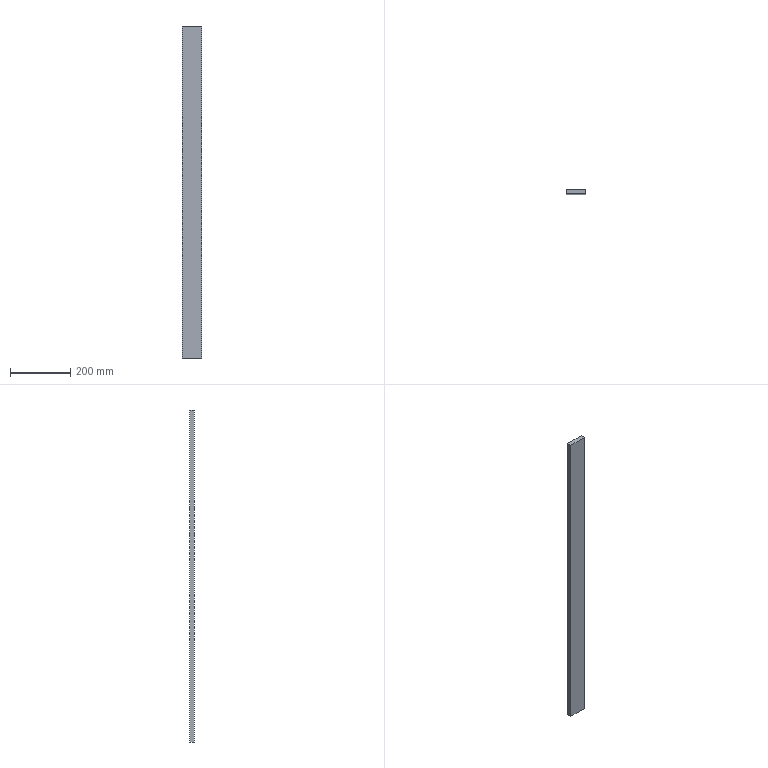Part | NX | features BREP 1 | 1 solid | 6 faces | box 65 x 15 x 1103 mm | volume 1075478 mm3 | plane 6
STEP:
#1=CARTESIAN_POINT('',(687.678,-679.988,1203.055));
#2=VERTEX_POINT('',#1);
#3=CARTESIAN_POINT('',(752.678,-679.988,1203.055));
#4=VERTEX_POINT('',#3);
#5=CARTESIAN_POINT('',(720.178,-679.988,1203.055));
#6=DIRECTION('',(1.,0.,0.));
#7=VECTOR('',#6,1000.);
#8=LINE('',#5,#7);
#9=EDGE_CURVE('',#2,#4,#8,.T.);
#10=ORIENTED_EDGE('',*,*,#9,.T.);
#11=CARTESIAN_POINT('',(752.678,-664.988,1203.055));
#12=VERTEX_POINT('',#11);
#13=CARTESIAN_POINT('',(752.678,-672.488,1203.055));
#14=DIRECTION('',(0.,1.,0.));
#15=VECTOR('',#14,1000.);
#16=LINE('',#13,#15);
#17=EDGE_CURVE('',#4,#12,#16,.T.);
#18=ORIENTED_EDGE('',*,*,#17,.T.);
#19=CARTESIAN_POINT('',(687.678,-664.988,1203.055));
#20=VERTEX_POINT('',#19);
#21=CARTESIAN_POINT('',(720.178,-664.988,1203.055));
#22=DIRECTION('',(1.,0.,0.));
#23=VECTOR('',#22,1000.);
#24=LINE('',#21,#23);
#25=EDGE_CURVE('',#20,#12,#24,.T.);
#26=ORIENTED_EDGE('',*,*,#25,.F.);
#27=CARTESIAN_POINT('',(687.678,-672.488,1203.055));
#28=DIRECTION('',(0.,1.,0.));
#29=VECTOR('',#28,1000.);
#30=LINE('',#27,#29);
#31=EDGE_CURVE('',#2,#20,#30,.T.);
#32=ORIENTED_EDGE('',*,*,#31,.F.);
#33=EDGE_LOOP('',(#10,#18,#26,#32));
#34=FACE_BOUND('',#33,.T.);
#35=CARTESIAN_POINT('',(717.678,-679.988,1203.055));
#36=DIRECTION('',(0.,0.,-1.));
#37=DIRECTION('',(1.,0.,0.));
#38=AXIS2_PLACEMENT_3D('',#35,#36,#37);
#39=PLANE('',#38);
#40=ADVANCED_FACE('',(#34),#39,.F.);
#41=CARTESIAN_POINT('',(687.678,-664.988,100.));
#42=VERTEX_POINT('',#41);
#43=CARTESIAN_POINT('',(687.678,-664.988,651.527));
#44=DIRECTION('',(0.,0.,-1.));
#45=VECTOR('',#44,1000.);
#46=LINE('',#43,#45);
#47=EDGE_CURVE('',#20,#42,#46,.T.);
#48=ORIENTED_EDGE('',*,*,#47,.F.);
#49=ORIENTED_EDGE('',*,*,#25,.T.);
#50=CARTESIAN_POINT('',(752.678,-664.988,100.));
#51=VERTEX_POINT('',#50);
#52=CARTESIAN_POINT('',(752.678,-664.988,651.527));
#53=DIRECTION('',(0.,0.,-1.));
#54=VECTOR('',#53,1000.);
#55=LINE('',#52,#54);
#56=EDGE_CURVE('',#12,#51,#55,.T.);
#57=ORIENTED_EDGE('',*,*,#56,.T.);
#58=CARTESIAN_POINT('',(720.178,-664.988,100.));
#59=DIRECTION('',(1.,0.,0.));
#60=VECTOR('',#59,1000.);
#61=LINE('',#58,#60);
#62=EDGE_CURVE('',#42,#51,#61,.T.);
#63=ORIENTED_EDGE('',*,*,#62,.F.);
#64=EDGE_LOOP('',(#48,#49,#57,#63));
#65=FACE_BOUND('',#64,.T.);
#66=CARTESIAN_POINT('',(1125.65,-664.988,1648.863));
#67=DIRECTION('',(0.,1.,0.));
#68=DIRECTION('',(-0.7071,0.,0.7071));
#69=AXIS2_PLACEMENT_3D('',#66,#67,#68);
#70=PLANE('',#69);
#71=ADVANCED_FACE('',(#65),#70,.T.);
#72=ORIENTED_EDGE('',*,*,#47,.T.);
#73=CARTESIAN_POINT('',(687.678,-679.988,100.));
#74=VERTEX_POINT('',#73);
#75=CARTESIAN_POINT('',(687.678,-672.488,100.));
#76=DIRECTION('',(0.,1.,0.));
#77=VECTOR('',#76,1000.);
#78=LINE('',#75,#77);
#79=EDGE_CURVE('',#74,#42,#78,.T.);
#80=ORIENTED_EDGE('',*,*,#79,.F.);
#81=CARTESIAN_POINT('',(687.678,-679.988,651.527));
#82=DIRECTION('',(0.,0.,-1.));
#83=VECTOR('',#82,1000.);
#84=LINE('',#81,#83);
#85=EDGE_CURVE('',#2,#74,#84,.T.);
#86=ORIENTED_EDGE('',*,*,#85,.F.);
#87=ORIENTED_EDGE('',*,*,#31,.T.);
#88=EDGE_LOOP('',(#72,#80,#86,#87));
#89=FACE_BOUND('',#88,.T.);
#90=CARTESIAN_POINT('',(687.678,-679.988,655.446));
#91=DIRECTION('',(-1.,0.,0.));
#92=DIRECTION('',(0.,1.,0.));
#93=AXIS2_PLACEMENT_3D('',#90,#91,#92);
#94=PLANE('',#93);
#95=ADVANCED_FACE('',(#89),#94,.T.);
#96=ORIENTED_EDGE('',*,*,#85,.T.);
#97=CARTESIAN_POINT('',(752.678,-679.988,100.));
#98=VERTEX_POINT('',#97);
#99=CARTESIAN_POINT('',(720.178,-679.988,100.));
#100=DIRECTION('',(1.,0.,0.));
#101=VECTOR('',#100,1000.);
#102=LINE('',#99,#101);
#103=EDGE_CURVE('',#74,#98,#102,.T.);
#104=ORIENTED_EDGE('',*,*,#103,.T.);
#105=CARTESIAN_POINT('',(752.678,-679.988,651.527));
#106=DIRECTION('',(0.,0.,-1.));
#107=VECTOR('',#106,1000.);
#108=LINE('',#105,#107);
#109=EDGE_CURVE('',#4,#98,#108,.T.);
#110=ORIENTED_EDGE('',*,*,#109,.F.);
#111=ORIENTED_EDGE('',*,*,#9,.F.);
#112=EDGE_LOOP('',(#96,#104,#110,#111));
#113=FACE_BOUND('',#112,.T.);
#114=CARTESIAN_POINT('',(1125.65,-679.988,1648.863));
#115=DIRECTION('',(0.,1.,0.));
#116=DIRECTION('',(-0.7071,0.,0.7071));
#117=AXIS2_PLACEMENT_3D('',#114,#115,#116);
#118=PLANE('',#117);
#119=ADVANCED_FACE('',(#113),#118,.F.);
#120=ORIENTED_EDGE('',*,*,#109,.T.);
#121=CARTESIAN_POINT('',(752.678,-672.488,100.));
#122=DIRECTION('',(0.,-1.,0.));
#123=VECTOR('',#122,1000.);
#124=LINE('',#121,#123);
#125=EDGE_CURVE('',#51,#98,#124,.T.);
#126=ORIENTED_EDGE('',*,*,#125,.F.);
#127=ORIENTED_EDGE('',*,*,#56,.F.);
#128=ORIENTED_EDGE('',*,*,#17,.F.);
#129=EDGE_LOOP('',(#120,#126,#127,#128));
#130=FACE_BOUND('',#129,.T.);
#131=CARTESIAN_POINT('',(752.678,-679.988,670.446));
#132=DIRECTION('',(-1.,0.,0.));
#133=DIRECTION('',(0.,1.,0.));
#134=AXIS2_PLACEMENT_3D('',#131,#132,#133);
#135=PLANE('',#134);
#136=ADVANCED_FACE('',(#130),#135,.F.);
#137=ORIENTED_EDGE('',*,*,#125,.T.);
#138=ORIENTED_EDGE('',*,*,#103,.F.);
#139=ORIENTED_EDGE('',*,*,#79,.T.);
#140=ORIENTED_EDGE('',*,*,#62,.T.);
#141=EDGE_LOOP('',(#137,#138,#139,#140));
#142=FACE_BOUND('',#141,.T.);
#143=CARTESIAN_POINT('',(702.678,-679.988,100.));
#144=DIRECTION('',(0.,0.,-1.));
#145=DIRECTION('',(1.,0.,0.));
#146=AXIS2_PLACEMENT_3D('',#143,#144,#145);
#147=PLANE('',#146);
#148=ADVANCED_FACE('',(#142),#147,.T.);
#149=CLOSED_SHELL('',(#40,#71,#95,#119,#136,#148));
#150=MANIFOLD_SOLID_BREP('',#149);
#151=(LENGTH_UNIT()NAMED_UNIT(*)SI_UNIT(.MILLI.,.METRE.));
#152=UNCERTAINTY_MEASURE_WITH_UNIT(LENGTH_MEASURE(0.00001),#151,'','');
#153=(NAMED_UNIT(*)PLANE_ANGLE_UNIT()SI_UNIT($,.RADIAN.));
#154=(NAMED_UNIT(*)SI_UNIT($,.STERADIAN.)SOLID_ANGLE_UNIT());
#155=(GEOMETRIC_REPRESENTATION_CONTEXT(3)GLOBAL_UNCERTAINTY_ASSIGNED_CONTEXT((#152))GLOBAL_UNIT_ASSIGNED_CONTEXT((#151,#153,#154))REPRESENTATION_CONTEXT('',''));
#156=ADVANCED_BREP_SHAPE_REPRESENTATION('',(#150),#155);